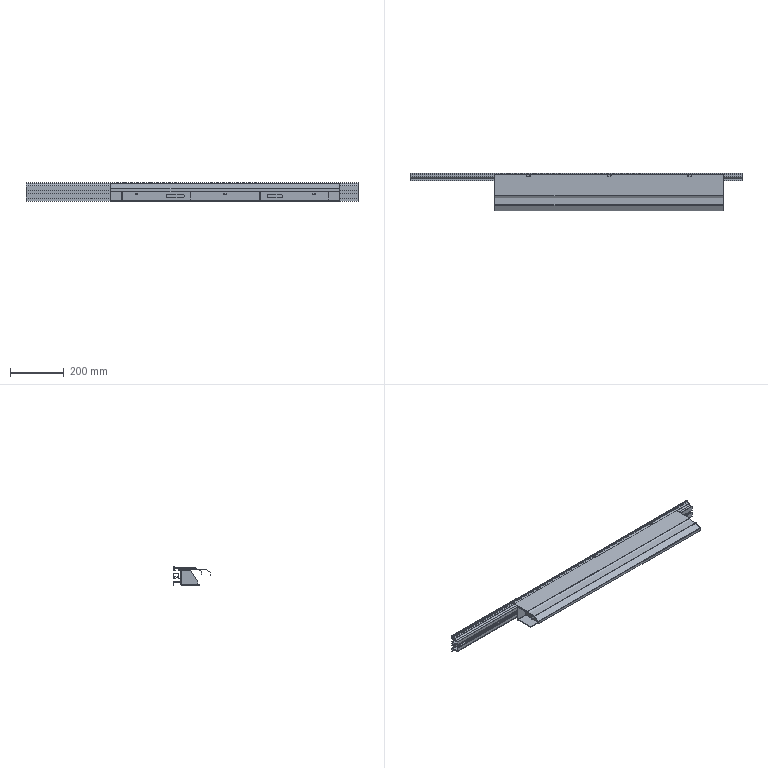Part | SolidWorks | 8 solids | 253 faces | box 1235 x 141.151 x 70 mm | volume 1052643 mm3 | plane 182 | cylinder 71 | commonest cylinder face diameters 10 x21 7 x18 2 x9 3 x7 6 x6 1 x4